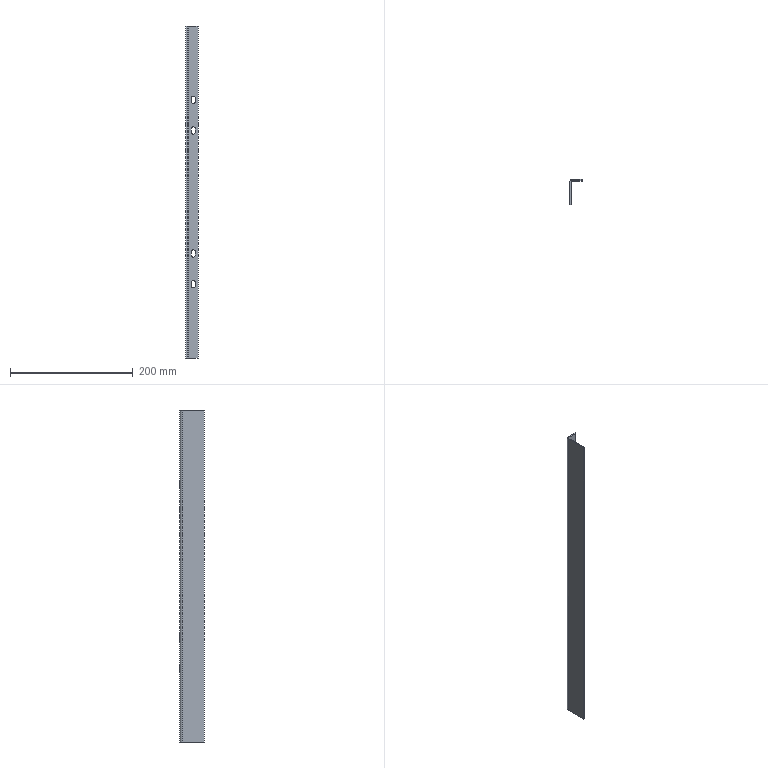Part | SolidWorks | features FlatPattern 1, ICE 1, SMBaseFlange 1, SheetMetal 1 | 1 solid | 34 faces | box 20 x 40 x 540 mm | volume 60662 mm3 | plane 20 | cylinder 14 | commonest cylinder face diameters 7 x12 4 x1 8 x1
STEP:
#1=CARTESIAN_POINT('',(12.,40.,114.));
#2=VERTEX_POINT('',#1);
#3=CARTESIAN_POINT('',(15.5,40.,117.5));
#4=VERTEX_POINT('',#3);
#5=CARTESIAN_POINT('',(12.,40.,117.5));
#6=DIRECTION('',(0.,-1.,0.));
#7=DIRECTION('',(0.,0.,-1.));
#8=AXIS2_PLACEMENT_3D('',#5,#6,#7);
#9=CIRCLE('',#8,3.5);
#10=EDGE_CURVE('',#2,#4,#9,.T.);
#11=ORIENTED_EDGE('',*,*,#10,.F.);
#12=CARTESIAN_POINT('',(12.,38.,114.));
#13=VERTEX_POINT('',#12);
#14=CARTESIAN_POINT('',(12.,40.,114.));
#15=DIRECTION('',(0.,-1.,0.));
#16=VECTOR('',#15,1000.);
#17=LINE('',#14,#16);
#18=EDGE_CURVE('',#2,#13,#17,.T.);
#19=ORIENTED_EDGE('',*,*,#18,.T.);
#20=CARTESIAN_POINT('',(15.5,38.,117.5));
#21=VERTEX_POINT('',#20);
#22=CARTESIAN_POINT('',(12.,38.,117.5));
#23=DIRECTION('',(0.,-1.,0.));
#24=DIRECTION('',(0.,0.,-1.));
#25=AXIS2_PLACEMENT_3D('',#22,#23,#24);
#26=CIRCLE('',#25,3.5);
#27=EDGE_CURVE('',#13,#21,#26,.T.);
#28=ORIENTED_EDGE('',*,*,#27,.T.);
#29=CARTESIAN_POINT('',(15.5,40.,117.5));
#30=DIRECTION('',(0.,-1.,0.));
#31=VECTOR('',#30,1000.);
#32=LINE('',#29,#31);
#33=EDGE_CURVE('',#4,#21,#32,.T.);
#34=ORIENTED_EDGE('',*,*,#33,.F.);
#35=EDGE_LOOP('',(#11,#19,#28,#34));
#36=FACE_OUTER_BOUND('',#35,.T.);
#37=CARTESIAN_POINT('',(12.,40.,117.5));
#38=DIRECTION('',(0.,-1.,0.));
#39=DIRECTION('',(0.,0.,-1.));
#40=AXIS2_PLACEMENT_3D('',#37,#38,#39);
#41=CYLINDRICAL_SURFACE('',#40,3.5);
#42=ADVANCED_FACE('',(#36),#41,.F.);
#43=CARTESIAN_POINT('',(12.,40.,164.));
#44=VERTEX_POINT('',#43);
#45=CARTESIAN_POINT('',(15.5,40.,167.5));
#46=VERTEX_POINT('',#45);
#47=CARTESIAN_POINT('',(12.,40.,167.5));
#48=DIRECTION('',(0.,-1.,0.));
#49=DIRECTION('',(0.,0.,-1.));
#50=AXIS2_PLACEMENT_3D('',#47,#48,#49);
#51=CIRCLE('',#50,3.5);
#52=EDGE_CURVE('',#44,#46,#51,.T.);
#53=ORIENTED_EDGE('',*,*,#52,.F.);
#54=CARTESIAN_POINT('',(12.,38.,164.));
#55=VERTEX_POINT('',#54);
#56=CARTESIAN_POINT('',(12.,40.,164.));
#57=DIRECTION('',(0.,-1.,0.));
#58=VECTOR('',#57,1000.);
#59=LINE('',#56,#58);
#60=EDGE_CURVE('',#44,#55,#59,.T.);
#61=ORIENTED_EDGE('',*,*,#60,.T.);
#62=CARTESIAN_POINT('',(15.5,38.,167.5));
#63=VERTEX_POINT('',#62);
#64=CARTESIAN_POINT('',(12.,38.,167.5));
#65=DIRECTION('',(0.,-1.,0.));
#66=DIRECTION('',(0.,0.,-1.));
#67=AXIS2_PLACEMENT_3D('',#64,#65,#66);
#68=CIRCLE('',#67,3.5);
#69=EDGE_CURVE('',#55,#63,#68,.T.);
#70=ORIENTED_EDGE('',*,*,#69,.T.);
#71=CARTESIAN_POINT('',(15.5,40.,167.5));
#72=DIRECTION('',(0.,-1.,0.));
#73=VECTOR('',#72,1000.);
#74=LINE('',#71,#73);
#75=EDGE_CURVE('',#46,#63,#74,.T.);
#76=ORIENTED_EDGE('',*,*,#75,.F.);
#77=EDGE_LOOP('',(#53,#61,#70,#76));
#78=FACE_OUTER_BOUND('',#77,.T.);
#79=CARTESIAN_POINT('',(12.,40.,167.5));
#80=DIRECTION('',(0.,-1.,0.));
#81=DIRECTION('',(0.,0.,-1.));
#82=AXIS2_PLACEMENT_3D('',#79,#80,#81);
#83=CYLINDRICAL_SURFACE('',#82,3.5);
#84=ADVANCED_FACE('',(#78),#83,.F.);
#85=CARTESIAN_POINT('',(12.,40.,364.));
#86=VERTEX_POINT('',#85);
#87=CARTESIAN_POINT('',(15.5,40.,367.5));
#88=VERTEX_POINT('',#87);
#89=CARTESIAN_POINT('',(12.,40.,367.5));
#90=DIRECTION('',(0.,-1.,0.));
#91=DIRECTION('',(0.,0.,1.));
#92=AXIS2_PLACEMENT_3D('',#89,#90,#91);
#93=CIRCLE('',#92,3.5);
#94=EDGE_CURVE('',#86,#88,#93,.T.);
#95=ORIENTED_EDGE('',*,*,#94,.F.);
#96=CARTESIAN_POINT('',(12.,38.,364.));
#97=VERTEX_POINT('',#96);
#98=CARTESIAN_POINT('',(12.,40.,364.));
#99=DIRECTION('',(0.,-1.,0.));
#100=VECTOR('',#99,1000.);
#101=LINE('',#98,#100);
#102=EDGE_CURVE('',#86,#97,#101,.T.);
#103=ORIENTED_EDGE('',*,*,#102,.T.);
#104=CARTESIAN_POINT('',(15.5,38.,367.5));
#105=VERTEX_POINT('',#104);
#106=CARTESIAN_POINT('',(12.,38.,367.5));
#107=DIRECTION('',(0.,-1.,0.));
#108=DIRECTION('',(0.,0.,1.));
#109=AXIS2_PLACEMENT_3D('',#106,#107,#108);
#110=CIRCLE('',#109,3.5);
#111=EDGE_CURVE('',#97,#105,#110,.T.);
#112=ORIENTED_EDGE('',*,*,#111,.T.);
#113=CARTESIAN_POINT('',(15.5,40.,367.5));
#114=DIRECTION('',(0.,-1.,0.));
#115=VECTOR('',#114,1000.);
#116=LINE('',#113,#115);
#117=EDGE_CURVE('',#88,#105,#116,.T.);
#118=ORIENTED_EDGE('',*,*,#117,.F.);
#119=EDGE_LOOP('',(#95,#103,#112,#118));
#120=FACE_OUTER_BOUND('',#119,.T.);
#121=CARTESIAN_POINT('',(12.,40.,367.5));
#122=DIRECTION('',(0.,-1.,0.));
#123=DIRECTION('',(0.,0.,-1.));
#124=AXIS2_PLACEMENT_3D('',#121,#122,#123);
#125=CYLINDRICAL_SURFACE('',#124,3.5);
#126=ADVANCED_FACE('',(#120),#125,.F.);
#127=CARTESIAN_POINT('',(12.,40.,414.));
#128=VERTEX_POINT('',#127);
#129=CARTESIAN_POINT('',(15.5,40.,417.5));
#130=VERTEX_POINT('',#129);
#131=CARTESIAN_POINT('',(12.,40.,417.5));
#132=DIRECTION('',(0.,-1.,0.));
#133=DIRECTION('',(0.,0.,1.));
#134=AXIS2_PLACEMENT_3D('',#131,#132,#133);
#135=CIRCLE('',#134,3.5);
#136=EDGE_CURVE('',#128,#130,#135,.T.);
#137=ORIENTED_EDGE('',*,*,#136,.F.);
#138=CARTESIAN_POINT('',(12.,38.,414.));
#139=VERTEX_POINT('',#138);
#140=CARTESIAN_POINT('',(12.,40.,414.));
#141=DIRECTION('',(0.,-1.,0.));
#142=VECTOR('',#141,1000.);
#143=LINE('',#140,#142);
#144=EDGE_CURVE('',#128,#139,#143,.T.);
#145=ORIENTED_EDGE('',*,*,#144,.T.);
#146=CARTESIAN_POINT('',(15.5,38.,417.5));
#147=VERTEX_POINT('',#146);
#148=CARTESIAN_POINT('',(12.,38.,417.5));
#149=DIRECTION('',(0.,-1.,0.));
#150=DIRECTION('',(0.,0.,1.));
#151=AXIS2_PLACEMENT_3D('',#148,#149,#150);
#152=CIRCLE('',#151,3.5);
#153=EDGE_CURVE('',#139,#147,#152,.T.);
#154=ORIENTED_EDGE('',*,*,#153,.T.);
#155=CARTESIAN_POINT('',(15.5,40.,417.5));
#156=DIRECTION('',(0.,-1.,0.));
#157=VECTOR('',#156,1000.);
#158=LINE('',#155,#157);
#159=EDGE_CURVE('',#130,#147,#158,.T.);
#160=ORIENTED_EDGE('',*,*,#159,.F.);
#161=EDGE_LOOP('',(#137,#145,#154,#160));
#162=FACE_OUTER_BOUND('',#161,.T.);
#163=CARTESIAN_POINT('',(12.,40.,417.5));
#164=DIRECTION('',(0.,-1.,0.));
#165=DIRECTION('',(0.,0.,-1.));
#166=AXIS2_PLACEMENT_3D('',#163,#164,#165);
#167=CYLINDRICAL_SURFACE('',#166,3.5);
#168=ADVANCED_FACE('',(#162),#167,.F.);
#169=CARTESIAN_POINT('',(4.,40.,540.));
#170=VERTEX_POINT('',#169);
#171=CARTESIAN_POINT('',(4.,38.,540.));
#172=VERTEX_POINT('',#171);
#173=CARTESIAN_POINT('',(4.,40.,540.));
#174=DIRECTION('',(0.,-1.,0.));
#175=VECTOR('',#174,1000.);
#176=LINE('',#173,#175);
#177=EDGE_CURVE('',#170,#172,#176,.T.);
#178=ORIENTED_EDGE('',*,*,#177,.F.);
#179=CARTESIAN_POINT('',(0.,36.,540.));
#180=VERTEX_POINT('',#179);
#181=CARTESIAN_POINT('',(4.,36.,540.));
#182=DIRECTION('',(0.,0.,-1.));
#183=DIRECTION('',(1.,0.,0.));
#184=AXIS2_PLACEMENT_3D('',#181,#182,#183);
#185=CIRCLE('',#184,4.);
#186=EDGE_CURVE('',#180,#170,#185,.T.);
#187=ORIENTED_EDGE('',*,*,#186,.F.);
#188=CARTESIAN_POINT('',(2.,36.,540.));
#189=VERTEX_POINT('',#188);
#190=CARTESIAN_POINT('',(2.,36.,540.));
#191=DIRECTION('',(-1.,0.,0.));
#192=VECTOR('',#191,1000.);
#193=LINE('',#190,#192);
#194=EDGE_CURVE('',#189,#180,#193,.T.);
#195=ORIENTED_EDGE('',*,*,#194,.F.);
#196=CARTESIAN_POINT('',(4.,36.,540.));
#197=DIRECTION('',(0.,0.,-1.));
#198=DIRECTION('',(1.,0.,0.));
#199=AXIS2_PLACEMENT_3D('',#196,#197,#198);
#200=CIRCLE('',#199,2.);
#201=EDGE_CURVE('',#189,#172,#200,.T.);
#202=ORIENTED_EDGE('',*,*,#201,.T.);
#203=EDGE_LOOP('',(#178,#187,#195,#202));
#204=FACE_OUTER_BOUND('',#203,.T.);
#205=CARTESIAN_POINT('',(4.,40.,540.));
#206=DIRECTION('',(0.,0.,1.));
#207=DIRECTION('',(1.,0.,0.));
#208=AXIS2_PLACEMENT_3D('',#205,#206,#207);
#209=PLANE('',#208);
#210=ADVANCED_FACE('',(#204),#209,.T.);
#211=CARTESIAN_POINT('',(20.,40.,540.));
#212=VERTEX_POINT('',#211);
#213=CARTESIAN_POINT('',(0.,40.,540.));
#214=DIRECTION('',(1.,0.,0.));
#215=VECTOR('',#214,1000.);
#216=LINE('',#213,#215);
#217=EDGE_CURVE('',#170,#212,#216,.T.);
#218=ORIENTED_EDGE('',*,*,#217,.F.);
#219=ORIENTED_EDGE('',*,*,#177,.T.);
#220=CARTESIAN_POINT('',(20.,38.,540.));
#221=VERTEX_POINT('',#220);
#222=CARTESIAN_POINT('',(0.,38.,540.));
#223=DIRECTION('',(1.,0.,0.));
#224=VECTOR('',#223,1000.);
#225=LINE('',#222,#224);
#226=EDGE_CURVE('',#172,#221,#225,.T.);
#227=ORIENTED_EDGE('',*,*,#226,.T.);
#228=CARTESIAN_POINT('',(20.,40.,540.));
#229=DIRECTION('',(0.,-1.,0.));
#230=VECTOR('',#229,1000.);
#231=LINE('',#228,#230);
#232=EDGE_CURVE('',#212,#221,#231,.T.);
#233=ORIENTED_EDGE('',*,*,#232,.F.);
#234=EDGE_LOOP('',(#218,#219,#227,#233));
#235=FACE_OUTER_BOUND('',#234,.T.);
#236=CARTESIAN_POINT('',(2.,36.,540.));
#237=DIRECTION('',(0.,0.,1.));
#238=DIRECTION('',(1.,0.,0.));
#239=AXIS2_PLACEMENT_3D('',#236,#237,#238);
#240=PLANE('',#239);
#241=ADVANCED_FACE('',(#235),#240,.T.);
#242=CARTESIAN_POINT('',(0.,36.,0.));
#243=VERTEX_POINT('',#242);
#244=CARTESIAN_POINT('',(2.,36.,0.));
#245=VERTEX_POINT('',#244);
#246=CARTESIAN_POINT('',(0.,36.,0.));
#247=DIRECTION('',(1.,0.,0.));
#248=VECTOR('',#247,1000.);
#249=LINE('',#246,#248);
#250=EDGE_CURVE('',#243,#245,#249,.T.);
#251=ORIENTED_EDGE('',*,*,#250,.F.);
#252=CARTESIAN_POINT('',(4.,40.,0.));
#253=VERTEX_POINT('',#252);
#254=CARTESIAN_POINT('',(4.,36.,0.));
#255=DIRECTION('',(0.,0.,-1.));
#256=DIRECTION('',(1.,0.,0.));
#257=AXIS2_PLACEMENT_3D('',#254,#255,#256);
#258=CIRCLE('',#257,4.);
#259=EDGE_CURVE('',#243,#253,#258,.T.);
#260=ORIENTED_EDGE('',*,*,#259,.T.);
#261=CARTESIAN_POINT('',(4.,38.,0.));
#262=VERTEX_POINT('',#261);
#263=CARTESIAN_POINT('',(4.,38.,0.));
#264=DIRECTION('',(0.,1.,0.));
#265=VECTOR('',#264,1000.);
#266=LINE('',#263,#265);
#267=EDGE_CURVE('',#262,#253,#266,.T.);
#268=ORIENTED_EDGE('',*,*,#267,.F.);
#269=CARTESIAN_POINT('',(4.,36.,0.));
#270=DIRECTION('',(0.,0.,-1.));
#271=DIRECTION('',(1.,0.,0.));
#272=AXIS2_PLACEMENT_3D('',#269,#270,#271);
#273=CIRCLE('',#272,2.);
#274=EDGE_CURVE('',#245,#262,#273,.T.);
#275=ORIENTED_EDGE('',*,*,#274,.F.);
#276=EDGE_LOOP('',(#251,#260,#268,#275));
#277=FACE_OUTER_BOUND('',#276,.T.);
#278=CARTESIAN_POINT('',(0.,36.,0.));
#279=DIRECTION('',(0.,0.,-1.));
#280=DIRECTION('',(-1.,0.,0.));
#281=AXIS2_PLACEMENT_3D('',#278,#279,#280);
#282=PLANE('',#281);
#283=ADVANCED_FACE('',(#277),#282,.T.);
#284=CARTESIAN_POINT('',(0.,0.,0.));
#285=VERTEX_POINT('',#284);
#286=CARTESIAN_POINT('',(0.,0.,0.));
#287=DIRECTION('',(0.,1.,0.));
#288=VECTOR('',#287,1000.);
#289=LINE('',#286,#288);
#290=EDGE_CURVE('',#285,#243,#289,.T.);
#291=ORIENTED_EDGE('',*,*,#290,.T.);
#292=ORIENTED_EDGE('',*,*,#250,.T.);
#293=CARTESIAN_POINT('',(2.,0.,0.));
#294=VERTEX_POINT('',#293);
#295=CARTESIAN_POINT('',(2.,0.,0.));
#296=DIRECTION('',(0.,1.,0.));
#297=VECTOR('',#296,1000.);
#298=LINE('',#295,#297);
#299=EDGE_CURVE('',#294,#245,#298,.T.);
#300=ORIENTED_EDGE('',*,*,#299,.F.);
#301=CARTESIAN_POINT('',(2.,0.,0.));
#302=DIRECTION('',(-1.,0.,0.));
#303=VECTOR('',#302,1000.);
#304=LINE('',#301,#303);
#305=EDGE_CURVE('',#294,#285,#304,.T.);
#306=ORIENTED_EDGE('',*,*,#305,.T.);
#307=EDGE_LOOP('',(#291,#292,#300,#306));
#308=FACE_OUTER_BOUND('',#307,.T.);
#309=CARTESIAN_POINT('',(4.,38.,0.));
#310=DIRECTION('',(0.,0.,-1.));
#311=DIRECTION('',(-1.,0.,0.));
#312=AXIS2_PLACEMENT_3D('',#309,#310,#311);
#313=PLANE('',#312);
#314=ADVANCED_FACE('',(#308),#313,.T.);
#315=CARTESIAN_POINT('',(15.5,38.,122.5));
#316=VERTEX_POINT('',#315);
#317=CARTESIAN_POINT('',(15.5,38.,117.5));
#318=DIRECTION('',(0.,0.,1.));
#319=VECTOR('',#318,1000.);
#320=LINE('',#317,#319);
#321=EDGE_CURVE('',#21,#316,#320,.T.);
#322=ORIENTED_EDGE('',*,*,#321,.F.);
#323=ORIENTED_EDGE('',*,*,#27,.F.);
#324=CARTESIAN_POINT('',(8.5,38.,117.5));
#325=VERTEX_POINT('',#324);
#326=CARTESIAN_POINT('',(12.,38.,117.5));
#327=DIRECTION('',(0.,-1.,0.));
#328=DIRECTION('',(0.,0.,-1.));
#329=AXIS2_PLACEMENT_3D('',#326,#327,#328);
#330=CIRCLE('',#329,3.5);
#331=EDGE_CURVE('',#325,#13,#330,.T.);
#332=ORIENTED_EDGE('',*,*,#331,.F.);
#333=CARTESIAN_POINT('',(8.5,38.,122.5));
#334=VERTEX_POINT('',#333);
#335=CARTESIAN_POINT('',(8.5,38.,117.5));
#336=DIRECTION('',(0.,0.,-1.));
#337=VECTOR('',#336,1000.);
#338=LINE('',#335,#337);
#339=EDGE_CURVE('',#334,#325,#338,.T.);
#340=ORIENTED_EDGE('',*,*,#339,.F.);
#341=CARTESIAN_POINT('',(12.,38.,122.5));
#342=DIRECTION('',(0.,-1.,0.));
#343=DIRECTION('',(0.,0.,-1.));
#344=AXIS2_PLACEMENT_3D('',#341,#342,#343);
#345=CIRCLE('',#344,3.5);
#346=EDGE_CURVE('',#316,#334,#345,.T.);
#347=ORIENTED_EDGE('',*,*,#346,.F.);
#348=EDGE_LOOP('',(#322,#323,#332,#340,#347));
#349=FACE_BOUND('',#348,.T.);
#350=CARTESIAN_POINT('',(15.5,38.,172.5));
#351=VERTEX_POINT('',#350);
#352=CARTESIAN_POINT('',(15.5,38.,167.5));
#353=DIRECTION('',(0.,0.,1.));
#354=VECTOR('',#353,1000.);
#355=LINE('',#352,#354);
#356=EDGE_CURVE('',#63,#351,#355,.T.);
#357=ORIENTED_EDGE('',*,*,#356,.F.);
#358=ORIENTED_EDGE('',*,*,#69,.F.);
#359=CARTESIAN_POINT('',(8.5,38.,167.5));
#360=VERTEX_POINT('',#359);
#361=CARTESIAN_POINT('',(12.,38.,167.5));
#362=DIRECTION('',(0.,-1.,0.));
#363=DIRECTION('',(0.,0.,-1.));
#364=AXIS2_PLACEMENT_3D('',#361,#362,#363);
#365=CIRCLE('',#364,3.5);
#366=EDGE_CURVE('',#360,#55,#365,.T.);
#367=ORIENTED_EDGE('',*,*,#366,.F.);
#368=CARTESIAN_POINT('',(8.5,38.,172.5));
#369=VERTEX_POINT('',#368);
#370=CARTESIAN_POINT('',(8.5,38.,167.5));
#371=DIRECTION('',(0.,0.,-1.));
#372=VECTOR('',#371,1000.);
#373=LINE('',#370,#372);
#374=EDGE_CURVE('',#369,#360,#373,.T.);
#375=ORIENTED_EDGE('',*,*,#374,.F.);
#376=CARTESIAN_POINT('',(12.,38.,172.5));
#377=DIRECTION('',(0.,-1.,0.));
#378=DIRECTION('',(0.,0.,-1.));
#379=AXIS2_PLACEMENT_3D('',#376,#377,#378);
#380=CIRCLE('',#379,3.5);
#381=EDGE_CURVE('',#351,#369,#380,.T.);
#382=ORIENTED_EDGE('',*,*,#381,.F.);
#383=EDGE_LOOP('',(#357,#358,#367,#375,#382));
#384=FACE_BOUND('',#383,.T.);
#385=CARTESIAN_POINT('',(8.5,38.,372.5));
#386=VERTEX_POINT('',#385);
#387=CARTESIAN_POINT('',(8.5,38.,367.5));
#388=VERTEX_POINT('',#387);
#389=CARTESIAN_POINT('',(8.5,38.,372.5));
#390=DIRECTION('',(0.,0.,-1.));
#391=VECTOR('',#390,1000.);
#392=LINE('',#389,#391);
#393=EDGE_CURVE('',#386,#388,#392,.T.);
#394=ORIENTED_EDGE('',*,*,#393,.F.);
#395=CARTESIAN_POINT('',(15.5,38.,372.5));
#396=VERTEX_POINT('',#395);
#397=CARTESIAN_POINT('',(12.,38.,372.5));
#398=DIRECTION('',(0.,-1.,0.));
#399=DIRECTION('',(0.,0.,1.));
#400=AXIS2_PLACEMENT_3D('',#397,#398,#399);
#401=CIRCLE('',#400,3.5);
#402=EDGE_CURVE('',#396,#386,#401,.T.);
#403=ORIENTED_EDGE('',*,*,#402,.F.);
#404=CARTESIAN_POINT('',(15.5,38.,372.5));
#405=DIRECTION('',(0.,0.,1.));
#406=VECTOR('',#405,1000.);
#407=LINE('',#404,#406);
#408=EDGE_CURVE('',#105,#396,#407,.T.);
#409=ORIENTED_EDGE('',*,*,#408,.F.);
#410=ORIENTED_EDGE('',*,*,#111,.F.);
#411=CARTESIAN_POINT('',(12.,38.,367.5));
#412=DIRECTION('',(0.,-1.,0.));
#413=DIRECTION('',(0.,0.,1.));
#414=AXIS2_PLACEMENT_3D('',#411,#412,#413);
#415=CIRCLE('',#414,3.5);
#416=EDGE_CURVE('',#388,#97,#415,.T.);
#417=ORIENTED_EDGE('',*,*,#416,.F.);
#418=EDGE_LOOP('',(#394,#403,#409,#410,#417));
#419=FACE_BOUND('',#418,.T.);
#420=CARTESIAN_POINT('',(8.5,38.,422.5));
#421=VERTEX_POINT('',#420);
#422=CARTESIAN_POINT('',(8.5,38.,417.5));
#423=VERTEX_POINT('',#422);
#424=CARTESIAN_POINT('',(8.5,38.,422.5));
#425=DIRECTION('',(0.,0.,-1.));
#426=VECTOR('',#425,1000.);
#427=LINE('',#424,#426);
#428=EDGE_CURVE('',#421,#423,#427,.T.);
#429=ORIENTED_EDGE('',*,*,#428,.F.);
#430=CARTESIAN_POINT('',(15.5,38.,422.5));
#431=VERTEX_POINT('',#430);
#432=CARTESIAN_POINT('',(12.,38.,422.5));
#433=DIRECTION('',(0.,-1.,0.));
#434=DIRECTION('',(0.,0.,1.));
#435=AXIS2_PLACEMENT_3D('',#432,#433,#434);
#436=CIRCLE('',#435,3.5);
#437=EDGE_CURVE('',#431,#421,#436,.T.);
#438=ORIENTED_EDGE('',*,*,#437,.F.);
#439=CARTESIAN_POINT('',(15.5,38.,422.5));
#440=DIRECTION('',(0.,0.,1.));
#441=VECTOR('',#440,1000.);
#442=LINE('',#439,#441);
#443=EDGE_CURVE('',#147,#431,#442,.T.);
#444=ORIENTED_EDGE('',*,*,#443,.F.);
#445=ORIENTED_EDGE('',*,*,#153,.F.);
#446=CARTESIAN_POINT('',(12.,38.,417.5));
#447=DIRECTION('',(0.,-1.,0.));
#448=DIRECTION('',(0.,0.,1.));
#449=AXIS2_PLACEMENT_3D('',#446,#447,#448);
#450=CIRCLE('',#449,3.5);
#451=EDGE_CURVE('',#423,#139,#450,.T.);
#452=ORIENTED_EDGE('',*,*,#451,.F.);
#453=EDGE_LOOP('',(#429,#438,#444,#445,#452));
#454=FACE_BOUND('',#453,.T.);
#455=CARTESIAN_POINT('',(20.,38.,0.));
#456=VERTEX_POINT('',#455);
#457=CARTESIAN_POINT('',(0.,38.,0.));
#458=DIRECTION('',(1.,0.,0.));
#459=VECTOR('',#458,1000.);
#460=LINE('',#457,#459);
#461=EDGE_CURVE('',#262,#456,#460,.T.);
#462=ORIENTED_EDGE('',*,*,#461,.T.);
#463=CARTESIAN_POINT('',(20.,38.,540.));
#464=DIRECTION('',(0.,0.,-1.));
#465=VECTOR('',#464,1000.);
#466=LINE('',#463,#465);
#467=EDGE_CURVE('',#221,#456,#466,.T.);
#468=ORIENTED_EDGE('',*,*,#467,.F.);
#469=ORIENTED_EDGE('',*,*,#226,.F.);
#470=CARTESIAN_POINT('',(4.,38.,540.));
#471=DIRECTION('',(0.,0.,-1.));
#472=VECTOR('',#471,1000.);
#473=LINE('',#470,#472);
#474=EDGE_CURVE('',#172,#262,#473,.T.);
#475=ORIENTED_EDGE('',*,*,#474,.T.);
#476=EDGE_LOOP('',(#462,#468,#469,#475));
#477=FACE_OUTER_BOUND('',#476,.T.);
#478=CARTESIAN_POINT('',(0.,38.,540.));
#479=DIRECTION('',(0.,1.,0.));
#480=DIRECTION('',(0.,0.,1.));
#481=AXIS2_PLACEMENT_3D('',#478,#479,#480);
#482=PLANE('',#481);
#483=ADVANCED_FACE('',(#349,#384,#419,#454,#477),#482,.F.);
#484=CARTESIAN_POINT('',(20.,40.,0.));
#485=VERTEX_POINT('',#484);
#486=CARTESIAN_POINT('',(20.,40.,0.));
#487=DIRECTION('',(0.,-1.,0.));
#488=VECTOR('',#487,1000.);
#489=LINE('',#486,#488);
#490=EDGE_CURVE('',#485,#456,#489,.T.);
#491=ORIENTED_EDGE('',*,*,#490,.F.);
#492=CARTESIAN_POINT('',(20.,40.,540.));
#493=DIRECTION('',(0.,0.,-1.));
#494=VECTOR('',#493,1000.);
#495=LINE('',#492,#494);
#496=EDGE_CURVE('',#212,#485,#495,.T.);
#497=ORIENTED_EDGE('',*,*,#496,.F.);
#498=ORIENTED_EDGE('',*,*,#232,.T.);
#499=ORIENTED_EDGE('',*,*,#467,.T.);
#500=EDGE_LOOP('',(#491,#497,#498,#499));
#501=FACE_OUTER_BOUND('',#500,.T.);
#502=CARTESIAN_POINT('',(20.,40.,540.));
#503=DIRECTION('',(1.,0.,0.));
#504=DIRECTION('',(0.,0.,-1.));
#505=AXIS2_PLACEMENT_3D('',#502,#503,#504);
#506=PLANE('',#505);
#507=ADVANCED_FACE('',(#501),#506,.T.);
#508=CARTESIAN_POINT('',(8.5,40.,117.5));
#509=VERTEX_POINT('',#508);
#510=CARTESIAN_POINT('',(12.,40.,117.5));
#511=DIRECTION('',(0.,-1.,0.));
#512=DIRECTION('',(0.,0.,-1.));
#513=AXIS2_PLACEMENT_3D('',#510,#511,#512);
#514=CIRCLE('',#513,3.5);
#515=EDGE_CURVE('',#509,#2,#514,.T.);
#516=ORIENTED_EDGE('',*,*,#515,.T.);
#517=ORIENTED_EDGE('',*,*,#10,.T.);
#518=CARTESIAN_POINT('',(15.5,40.,122.5));
#519=VERTEX_POINT('',#518);
#520=CARTESIAN_POINT('',(15.5,40.,117.5));
#521=DIRECTION('',(0.,0.,1.));
#522=VECTOR('',#521,1000.);
#523=LINE('',#520,#522);
#524=EDGE_CURVE('',#4,#519,#523,.T.);
#525=ORIENTED_EDGE('',*,*,#524,.T.);
#526=CARTESIAN_POINT('',(8.5,40.,122.5));
#527=VERTEX_POINT('',#526);
#528=CARTESIAN_POINT('',(12.,40.,122.5));
#529=DIRECTION('',(0.,-1.,0.));
#530=DIRECTION('',(0.,0.,-1.));
#531=AXIS2_PLACEMENT_3D('',#528,#529,#530);
#532=CIRCLE('',#531,3.5);
#533=EDGE_CURVE('',#519,#527,#532,.T.);
#534=ORIENTED_EDGE('',*,*,#533,.T.);
#535=CARTESIAN_POINT('',(8.5,40.,117.5));
#536=DIRECTION('',(0.,0.,-1.));
#537=VECTOR('',#536,1000.);
#538=LINE('',#535,#537);
#539=EDGE_CURVE('',#527,#509,#538,.T.);
#540=ORIENTED_EDGE('',*,*,#539,.T.);
#541=EDGE_LOOP('',(#516,#517,#525,#534,#540));
#542=FACE_BOUND('',#541,.T.);
#543=CARTESIAN_POINT('',(8.5,40.,167.5));
#544=VERTEX_POINT('',#543);
#545=CARTESIAN_POINT('',(12.,40.,167.5));
#546=DIRECTION('',(0.,-1.,0.));
#547=DIRECTION('',(0.,0.,-1.));
#548=AXIS2_PLACEMENT_3D('',#545,#546,#547);
#549=CIRCLE('',#548,3.5);
#550=EDGE_CURVE('',#544,#44,#549,.T.);
#551=ORIENTED_EDGE('',*,*,#550,.T.);
#552=ORIENTED_EDGE('',*,*,#52,.T.);
#553=CARTESIAN_POINT('',(15.5,40.,172.5));
#554=VERTEX_POINT('',#553);
#555=CARTESIAN_POINT('',(15.5,40.,167.5));
#556=DIRECTION('',(0.,0.,1.));
#557=VECTOR('',#556,1000.);
#558=LINE('',#555,#557);
#559=EDGE_CURVE('',#46,#554,#558,.T.);
#560=ORIENTED_EDGE('',*,*,#559,.T.);
#561=CARTESIAN_POINT('',(8.5,40.,172.5));
#562=VERTEX_POINT('',#561);
#563=CARTESIAN_POINT('',(12.,40.,172.5));
#564=DIRECTION('',(0.,-1.,0.));
#565=DIRECTION('',(0.,0.,-1.));
#566=AXIS2_PLACEMENT_3D('',#563,#564,#565);
#567=CIRCLE('',#566,3.5);
#568=EDGE_CURVE('',#554,#562,#567,.T.);
#569=ORIENTED_EDGE('',*,*,#568,.T.);
#570=CARTESIAN_POINT('',(8.5,40.,167.5));
#571=DIRECTION('',(0.,0.,-1.));
#572=VECTOR('',#571,1000.);
#573=LINE('',#570,#572);
#574=EDGE_CURVE('',#562,#544,#573,.T.);
#575=ORIENTED_EDGE('',*,*,#574,.T.);
#576=EDGE_LOOP('',(#551,#552,#560,#569,#575));
#577=FACE_BOUND('',#576,.T.);
#578=CARTESIAN_POINT('',(15.5,40.,372.5));
#579=VERTEX_POINT('',#578);
#580=CARTESIAN_POINT('',(8.5,40.,372.5));
#581=VERTEX_POINT('',#580);
#582=CARTESIAN_POINT('',(12.,40.,372.5));
#583=DIRECTION('',(0.,-1.,0.));
#584=DIRECTION('',(0.,0.,1.));
#585=AXIS2_PLACEMENT_3D('',#582,#583,#584);
#586=CIRCLE('',#585,3.5);
#587=EDGE_CURVE('',#579,#581,#586,.T.);
#588=ORIENTED_EDGE('',*,*,#587,.T.);
#589=CARTESIAN_POINT('',(8.5,40.,367.5));
#590=VERTEX_POINT('',#589);
#591=CARTESIAN_POINT('',(8.5,40.,372.5));
#592=DIRECTION('',(0.,0.,-1.));
#593=VECTOR('',#592,1000.);
#594=LINE('',#591,#593);
#595=EDGE_CURVE('',#581,#590,#594,.T.);
#596=ORIENTED_EDGE('',*,*,#595,.T.);
#597=CARTESIAN_POINT('',(12.,40.,367.5));
#598=DIRECTION('',(0.,-1.,0.));
#599=DIRECTION('',(0.,0.,1.));
#600=AXIS2_PLACEMENT_3D('',#597,#598,#599);
#601=CIRCLE('',#600,3.5);
#602=EDGE_CURVE('',#590,#86,#601,.T.);
#603=ORIENTED_EDGE('',*,*,#602,.T.);
#604=ORIENTED_EDGE('',*,*,#94,.T.);
#605=CARTESIAN_POINT('',(15.5,40.,372.5));
#606=DIRECTION('',(0.,0.,1.));
#607=VECTOR('',#606,1000.);
#608=LINE('',#605,#607);
#609=EDGE_CURVE('',#88,#579,#608,.T.);
#610=ORIENTED_EDGE('',*,*,#609,.T.);
#611=EDGE_LOOP('',(#588,#596,#603,#604,#610));
#612=FACE_BOUND('',#611,.T.);
#613=CARTESIAN_POINT('',(15.5,40.,422.5));
#614=VERTEX_POINT('',#613);
#615=CARTESIAN_POINT('',(8.5,40.,422.5));
#616=VERTEX_POINT('',#615);
#617=CARTESIAN_POINT('',(12.,40.,422.5));
#618=DIRECTION('',(0.,-1.,0.));
#619=DIRECTION('',(0.,0.,1.));
#620=AXIS2_PLACEMENT_3D('',#617,#618,#619);
#621=CIRCLE('',#620,3.5);
#622=EDGE_CURVE('',#614,#616,#621,.T.);
#623=ORIENTED_EDGE('',*,*,#622,.T.);
#624=CARTESIAN_POINT('',(8.5,40.,417.5));
#625=VERTEX_POINT('',#624);
#626=CARTESIAN_POINT('',(8.5,40.,422.5));
#627=DIRECTION('',(0.,0.,-1.));
#628=VECTOR('',#627,1000.);
#629=LINE('',#626,#628);
#630=EDGE_CURVE('',#616,#625,#629,.T.);
#631=ORIENTED_EDGE('',*,*,#630,.T.);
#632=CARTESIAN_POINT('',(12.,40.,417.5));
#633=DIRECTION('',(0.,-1.,0.));
#634=DIRECTION('',(0.,0.,1.));
#635=AXIS2_PLACEMENT_3D('',#632,#633,#634);
#636=CIRCLE('',#635,3.5);
#637=EDGE_CURVE('',#625,#128,#636,.T.);
#638=ORIENTED_EDGE('',*,*,#637,.T.);
#639=ORIENTED_EDGE('',*,*,#136,.T.);
#640=CARTESIAN_POINT('',(15.5,40.,422.5));
#641=DIRECTION('',(0.,0.,1.));
#642=VECTOR('',#641,1000.);
#643=LINE('',#640,#642);
#644=EDGE_CURVE('',#130,#614,#643,.T.);
#645=ORIENTED_EDGE('',*,*,#644,.T.);
#646=EDGE_LOOP('',(#623,#631,#638,#639,#645));
#647=FACE_BOUND('',#646,.T.);
#648=CARTESIAN_POINT('',(0.,40.,0.));
#649=DIRECTION('',(1.,0.,0.));
#650=VECTOR('',#649,1000.);
#651=LINE('',#648,#650);
#652=EDGE_CURVE('',#253,#485,#651,.T.);
#653=ORIENTED_EDGE('',*,*,#652,.F.);
#654=CARTESIAN_POINT('',(4.,40.,540.));
#655=DIRECTION('',(0.,0.,-1.));
#656=VECTOR('',#655,1000.);
#657=LINE('',#654,#656);
#658=EDGE_CURVE('',#170,#253,#657,.T.);
#659=ORIENTED_EDGE('',*,*,#658,.F.);
#660=ORIENTED_EDGE('',*,*,#217,.T.);
#661=ORIENTED_EDGE('',*,*,#496,.T.);
#662=EDGE_LOOP('',(#653,#659,#660,#661));
#663=FACE_OUTER_BOUND('',#662,.T.);
#664=CARTESIAN_POINT('',(0.,40.,540.));
#665=DIRECTION('',(0.,1.,0.));
#666=DIRECTION('',(0.,0.,1.));
#667=AXIS2_PLACEMENT_3D('',#664,#665,#666);
#668=PLANE('',#667);
#669=ADVANCED_FACE('',(#542,#577,#612,#647,#663),#668,.T.);
#670=ORIENTED_EDGE('',*,*,#259,.F.);
#671=CARTESIAN_POINT('',(0.,36.,540.));
#672=DIRECTION('',(0.,0.,-1.));
#673=VECTOR('',#672,1000.);
#674=LINE('',#671,#673);
#675=EDGE_CURVE('',#180,#243,#674,.T.);
#676=ORIENTED_EDGE('',*,*,#675,.F.);
#677=ORIENTED_EDGE('',*,*,#186,.T.);
#678=ORIENTED_EDGE('',*,*,#658,.T.);
#679=EDGE_LOOP('',(#670,#676,#677,#678));
#680=FACE_OUTER_BOUND('',#679,.T.);
#681=CARTESIAN_POINT('',(4.,36.,540.));
#682=DIRECTION('',(0.,0.,-1.));
#683=DIRECTION('',(-1.,0.,0.));
#684=AXIS2_PLACEMENT_3D('',#681,#682,#683);
#685=CYLINDRICAL_SURFACE('',#684,4.);
#686=ADVANCED_FACE('',(#680),#685,.T.);
#687=ORIENTED_EDGE('',*,*,#290,.F.);
#688=CARTESIAN_POINT('',(0.,0.,540.));
#689=VERTEX_POINT('',#688);
#690=CARTESIAN_POINT('',(0.,0.,540.));
#691=DIRECTION('',(0.,0.,-1.));
#692=VECTOR('',#691,1000.);
#693=LINE('',#690,#692);
#694=EDGE_CURVE('',#689,#285,#693,.T.);
#695=ORIENTED_EDGE('',*,*,#694,.F.);
#696=CARTESIAN_POINT('',(0.,0.,540.));
#697=DIRECTION('',(0.,1.,0.));
#698=VECTOR('',#697,1000.);
#699=LINE('',#696,#698);
#700=EDGE_CURVE('',#689,#180,#699,.T.);
#701=ORIENTED_EDGE('',*,*,#700,.T.);
#702=ORIENTED_EDGE('',*,*,#675,.T.);
#703=EDGE_LOOP('',(#687,#695,#701,#702));
#704=FACE_OUTER_BOUND('',#703,.T.);
#705=CARTESIAN_POINT('',(0.,0.,540.));
#706=DIRECTION('',(-1.,0.,0.));
#707=DIRECTION('',(0.,0.,1.));
#708=AXIS2_PLACEMENT_3D('',#705,#706,#707);
#709=PLANE('',#708);
#710=ADVANCED_FACE('',(#704),#709,.T.);
#711=ORIENTED_EDGE('',*,*,#305,.F.);
#712=CARTESIAN_POINT('',(2.,0.,540.));
#713=VERTEX_POINT('',#712);
#714=CARTESIAN_POINT('',(2.,0.,540.));
#715=DIRECTION('',(0.,0.,-1.));
#716=VECTOR('',#715,1000.);
#717=LINE('',#714,#716);
#718=EDGE_CURVE('',#713,#294,#717,.T.);
#719=ORIENTED_EDGE('',*,*,#718,.F.);
#720=CARTESIAN_POINT('',(2.,0.,540.));
#721=DIRECTION('',(-1.,0.,0.));
#722=VECTOR('',#721,1000.);
#723=LINE('',#720,#722);
#724=EDGE_CURVE('',#713,#689,#723,.T.);
#725=ORIENTED_EDGE('',*,*,#724,.T.);
#726=ORIENTED_EDGE('',*,*,#694,.T.);
#727=EDGE_LOOP('',(#711,#719,#725,#726));
#728=FACE_OUTER_BOUND('',#727,.T.);
#729=CARTESIAN_POINT('',(2.,0.,540.));
#730=DIRECTION('',(0.,-1.,0.));
#731=DIRECTION('',(0.,0.,-1.));
#732=AXIS2_PLACEMENT_3D('',#729,#730,#731);
#733=PLANE('',#732);
#734=ADVANCED_FACE('',(#728),#733,.T.);
#735=ORIENTED_EDGE('',*,*,#299,.T.);
#736=CARTESIAN_POINT('',(2.,36.,540.));
#737=DIRECTION('',(0.,0.,-1.));
#738=VECTOR('',#737,1000.);
#739=LINE('',#736,#738);
#740=EDGE_CURVE('',#189,#245,#739,.T.);
#741=ORIENTED_EDGE('',*,*,#740,.F.);
#742=CARTESIAN_POINT('',(2.,0.,540.));
#743=DIRECTION('',(0.,1.,0.));
#744=VECTOR('',#743,1000.);
#745=LINE('',#742,#744);
#746=EDGE_CURVE('',#713,#189,#745,.T.);
#747=ORIENTED_EDGE('',*,*,#746,.F.);
#748=ORIENTED_EDGE('',*,*,#718,.T.);
#749=EDGE_LOOP('',(#735,#741,#747,#748));
#750=FACE_OUTER_BOUND('',#749,.T.);
#751=CARTESIAN_POINT('',(2.,0.,540.));
#752=DIRECTION('',(-1.,0.,0.));
#753=DIRECTION('',(0.,0.,1.));
#754=AXIS2_PLACEMENT_3D('',#751,#752,#753);
#755=PLANE('',#754);
#756=ADVANCED_FACE('',(#750),#755,.F.);
#757=ORIENTED_EDGE('',*,*,#274,.T.);
#758=ORIENTED_EDGE('',*,*,#474,.F.);
#759=ORIENTED_EDGE('',*,*,#201,.F.);
#760=ORIENTED_EDGE('',*,*,#740,.T.);
#761=EDGE_LOOP('',(#757,#758,#759,#760));
#762=FACE_OUTER_BOUND('',#761,.T.);
#763=CARTESIAN_POINT('',(4.,36.,540.));
#764=DIRECTION('',(0.,0.,-1.));
#765=DIRECTION('',(-1.,0.,0.));
#766=AXIS2_PLACEMENT_3D('',#763,#764,#765);
#767=CYLINDRICAL_SURFACE('',#766,2.);
#768=ADVANCED_FACE('',(#762),#767,.F.);
#769=ORIENTED_EDGE('',*,*,#746,.T.);
#770=ORIENTED_EDGE('',*,*,#194,.T.);
#771=ORIENTED_EDGE('',*,*,#700,.F.);
#772=ORIENTED_EDGE('',*,*,#724,.F.);
#773=EDGE_LOOP('',(#769,#770,#771,#772));
#774=FACE_OUTER_BOUND('',#773,.T.);
#775=CARTESIAN_POINT('',(4.,36.,540.));
#776=DIRECTION('',(0.,0.,1.));
#777=DIRECTION('',(1.,0.,0.));
#778=AXIS2_PLACEMENT_3D('',#775,#776,#777);
#779=PLANE('',#778);
#780=ADVANCED_FACE('',(#774),#779,.T.);
#781=ORIENTED_EDGE('',*,*,#461,.F.);
#782=ORIENTED_EDGE('',*,*,#267,.T.);
#783=ORIENTED_EDGE('',*,*,#652,.T.);
#784=ORIENTED_EDGE('',*,*,#490,.T.);
#785=EDGE_LOOP('',(#781,#782,#783,#784));
#786=FACE_OUTER_BOUND('',#785,.T.);
#787=CARTESIAN_POINT('',(4.,36.,0.));
#788=DIRECTION('',(0.,0.,1.));
#789=DIRECTION('',(1.,0.,0.));
#790=AXIS2_PLACEMENT_3D('',#787,#788,#789);
#791=PLANE('',#790);
#792=ADVANCED_FACE('',(#786),#791,.F.);
#793=ORIENTED_EDGE('',*,*,#437,.T.);
#794=CARTESIAN_POINT('',(8.5,40.,422.5));
#795=DIRECTION('',(0.,-1.,0.));
#796=VECTOR('',#795,1000.);
#797=LINE('',#794,#796);
#798=EDGE_CURVE('',#616,#421,#797,.T.);
#799=ORIENTED_EDGE('',*,*,#798,.F.);
#800=ORIENTED_EDGE('',*,*,#622,.F.);
#801=CARTESIAN_POINT('',(15.5,40.,422.5));
#802=DIRECTION('',(0.,-1.,0.));
#803=VECTOR('',#802,1000.);
#804=LINE('',#801,#803);
#805=EDGE_CURVE('',#614,#431,#804,.T.);
#806=ORIENTED_EDGE('',*,*,#805,.T.);
#807=EDGE_LOOP('',(#793,#799,#800,#806));
#808=FACE_OUTER_BOUND('',#807,.T.);
#809=CARTESIAN_POINT('',(12.,40.,422.5));
#810=DIRECTION('',(0.,-1.,0.));
#811=DIRECTION('',(0.,0.,-1.));
#812=AXIS2_PLACEMENT_3D('',#809,#810,#811);
#813=CYLINDRICAL_SURFACE('',#812,3.5);
#814=ADVANCED_FACE('',(#808),#813,.F.);
#815=ORIENTED_EDGE('',*,*,#443,.T.);
#816=ORIENTED_EDGE('',*,*,#805,.F.);
#817=ORIENTED_EDGE('',*,*,#644,.F.);
#818=ORIENTED_EDGE('',*,*,#159,.T.);
#819=EDGE_LOOP('',(#815,#816,#817,#818));
#820=FACE_OUTER_BOUND('',#819,.T.);
#821=CARTESIAN_POINT('',(15.5,40.,422.5));
#822=DIRECTION('',(1.,0.,0.));
#823=DIRECTION('',(0.,0.,-1.));
#824=AXIS2_PLACEMENT_3D('',#821,#822,#823);
#825=PLANE('',#824);
#826=ADVANCED_FACE('',(#820),#825,.F.);
#827=ORIENTED_EDGE('',*,*,#144,.F.);
#828=ORIENTED_EDGE('',*,*,#637,.F.);
#829=CARTESIAN_POINT('',(8.5,40.,417.5));
#830=DIRECTION('',(0.,-1.,0.));
#831=VECTOR('',#830,1000.);
#832=LINE('',#829,#831);
#833=EDGE_CURVE('',#625,#423,#832,.T.);
#834=ORIENTED_EDGE('',*,*,#833,.T.);
#835=ORIENTED_EDGE('',*,*,#451,.T.);
#836=EDGE_LOOP('',(#827,#828,#834,#835));
#837=FACE_OUTER_BOUND('',#836,.T.);
#838=CARTESIAN_POINT('',(12.,40.,417.5));
#839=DIRECTION('',(0.,-1.,0.));
#840=DIRECTION('',(0.,0.,-1.));
#841=AXIS2_PLACEMENT_3D('',#838,#839,#840);
#842=CYLINDRICAL_SURFACE('',#841,3.5);
#843=ADVANCED_FACE('',(#837),#842,.F.);
#844=ORIENTED_EDGE('',*,*,#428,.T.);
#845=ORIENTED_EDGE('',*,*,#833,.F.);
#846=ORIENTED_EDGE('',*,*,#630,.F.);
#847=ORIENTED_EDGE('',*,*,#798,.T.);
#848=EDGE_LOOP('',(#844,#845,#846,#847));
#849=FACE_OUTER_BOUND('',#848,.T.);
#850=CARTESIAN_POINT('',(8.5,40.,422.5));
#851=DIRECTION('',(-1.,0.,0.));
#852=DIRECTION('',(0.,0.,1.));
#853=AXIS2_PLACEMENT_3D('',#850,#851,#852);
#854=PLANE('',#853);
#855=ADVANCED_FACE('',(#849),#854,.F.);
#856=ORIENTED_EDGE('',*,*,#402,.T.);
#857=CARTESIAN_POINT('',(8.5,40.,372.5));
#858=DIRECTION('',(0.,-1.,0.));
#859=VECTOR('',#858,1000.);
#860=LINE('',#857,#859);
#861=EDGE_CURVE('',#581,#386,#860,.T.);
#862=ORIENTED_EDGE('',*,*,#861,.F.);
#863=ORIENTED_EDGE('',*,*,#587,.F.);
#864=CARTESIAN_POINT('',(15.5,40.,372.5));
#865=DIRECTION('',(0.,-1.,0.));
#866=VECTOR('',#865,1000.);
#867=LINE('',#864,#866);
#868=EDGE_CURVE('',#579,#396,#867,.T.);
#869=ORIENTED_EDGE('',*,*,#868,.T.);
#870=EDGE_LOOP('',(#856,#862,#863,#869));
#871=FACE_OUTER_BOUND('',#870,.T.);
#872=CARTESIAN_POINT('',(12.,40.,372.5));
#873=DIRECTION('',(0.,-1.,0.));
#874=DIRECTION('',(0.,0.,-1.));
#875=AXIS2_PLACEMENT_3D('',#872,#873,#874);
#876=CYLINDRICAL_SURFACE('',#875,3.5);
#877=ADVANCED_FACE('',(#871),#876,.F.);
#878=ORIENTED_EDGE('',*,*,#408,.T.);
#879=ORIENTED_EDGE('',*,*,#868,.F.);
#880=ORIENTED_EDGE('',*,*,#609,.F.);
#881=ORIENTED_EDGE('',*,*,#117,.T.);
#882=EDGE_LOOP('',(#878,#879,#880,#881));
#883=FACE_OUTER_BOUND('',#882,.T.);
#884=CARTESIAN_POINT('',(15.5,40.,372.5));
#885=DIRECTION('',(1.,0.,0.));
#886=DIRECTION('',(0.,0.,-1.));
#887=AXIS2_PLACEMENT_3D('',#884,#885,#886);
#888=PLANE('',#887);
#889=ADVANCED_FACE('',(#883),#888,.F.);
#890=ORIENTED_EDGE('',*,*,#102,.F.);
#891=ORIENTED_EDGE('',*,*,#602,.F.);
#892=CARTESIAN_POINT('',(8.5,40.,367.5));
#893=DIRECTION('',(0.,-1.,0.));
#894=VECTOR('',#893,1000.);
#895=LINE('',#892,#894);
#896=EDGE_CURVE('',#590,#388,#895,.T.);
#897=ORIENTED_EDGE('',*,*,#896,.T.);
#898=ORIENTED_EDGE('',*,*,#416,.T.);
#899=EDGE_LOOP('',(#890,#891,#897,#898));
#900=FACE_OUTER_BOUND('',#899,.T.);
#901=CARTESIAN_POINT('',(12.,40.,367.5));
#902=DIRECTION('',(0.,-1.,0.));
#903=DIRECTION('',(0.,0.,-1.));
#904=AXIS2_PLACEMENT_3D('',#901,#902,#903);
#905=CYLINDRICAL_SURFACE('',#904,3.5);
#906=ADVANCED_FACE('',(#900),#905,.F.);
#907=ORIENTED_EDGE('',*,*,#393,.T.);
#908=ORIENTED_EDGE('',*,*,#896,.F.);
#909=ORIENTED_EDGE('',*,*,#595,.F.);
#910=ORIENTED_EDGE('',*,*,#861,.T.);
#911=EDGE_LOOP('',(#907,#908,#909,#910));
#912=FACE_OUTER_BOUND('',#911,.T.);
#913=CARTESIAN_POINT('',(8.5,40.,372.5));
#914=DIRECTION('',(-1.,0.,0.));
#915=DIRECTION('',(0.,0.,1.));
#916=AXIS2_PLACEMENT_3D('',#913,#914,#915);
#917=PLANE('',#916);
#918=ADVANCED_FACE('',(#912),#917,.F.);
#919=ORIENTED_EDGE('',*,*,#60,.F.);
#920=ORIENTED_EDGE('',*,*,#550,.F.);
#921=CARTESIAN_POINT('',(8.5,40.,167.5));
#922=DIRECTION('',(0.,-1.,0.));
#923=VECTOR('',#922,1000.);
#924=LINE('',#921,#923);
#925=EDGE_CURVE('',#544,#360,#924,.T.);
#926=ORIENTED_EDGE('',*,*,#925,.T.);
#927=ORIENTED_EDGE('',*,*,#366,.T.);
#928=EDGE_LOOP('',(#919,#920,#926,#927));
#929=FACE_OUTER_BOUND('',#928,.T.);
#930=CARTESIAN_POINT('',(12.,40.,167.5));
#931=DIRECTION('',(0.,-1.,0.));
#932=DIRECTION('',(0.,0.,-1.));
#933=AXIS2_PLACEMENT_3D('',#930,#931,#932);
#934=CYLINDRICAL_SURFACE('',#933,3.5);
#935=ADVANCED_FACE('',(#929),#934,.F.);
#936=ORIENTED_EDGE('',*,*,#374,.T.);
#937=ORIENTED_EDGE('',*,*,#925,.F.);
#938=ORIENTED_EDGE('',*,*,#574,.F.);
#939=CARTESIAN_POINT('',(8.5,40.,172.5));
#940=DIRECTION('',(0.,-1.,0.));
#941=VECTOR('',#940,1000.);
#942=LINE('',#939,#941);
#943=EDGE_CURVE('',#562,#369,#942,.T.);
#944=ORIENTED_EDGE('',*,*,#943,.T.);
#945=EDGE_LOOP('',(#936,#937,#938,#944));
#946=FACE_OUTER_BOUND('',#945,.T.);
#947=CARTESIAN_POINT('',(8.5,40.,167.5));
#948=DIRECTION('',(-1.,0.,0.));
#949=DIRECTION('',(0.,0.,1.));
#950=AXIS2_PLACEMENT_3D('',#947,#948,#949);
#951=PLANE('',#950);
#952=ADVANCED_FACE('',(#946),#951,.F.);
#953=ORIENTED_EDGE('',*,*,#381,.T.);
#954=ORIENTED_EDGE('',*,*,#943,.F.);
#955=ORIENTED_EDGE('',*,*,#568,.F.);
#956=CARTESIAN_POINT('',(15.5,40.,172.5));
#957=DIRECTION('',(0.,-1.,0.));
#958=VECTOR('',#957,1000.);
#959=LINE('',#956,#958);
#960=EDGE_CURVE('',#554,#351,#959,.T.);
#961=ORIENTED_EDGE('',*,*,#960,.T.);
#962=EDGE_LOOP('',(#953,#954,#955,#961));
#963=FACE_OUTER_BOUND('',#962,.T.);
#964=CARTESIAN_POINT('',(12.,40.,172.5));
#965=DIRECTION('',(0.,-1.,0.));
#966=DIRECTION('',(0.,0.,-1.));
#967=AXIS2_PLACEMENT_3D('',#964,#965,#966);
#968=CYLINDRICAL_SURFACE('',#967,3.5);
#969=ADVANCED_FACE('',(#963),#968,.F.);
#970=ORIENTED_EDGE('',*,*,#356,.T.);
#971=ORIENTED_EDGE('',*,*,#960,.F.);
#972=ORIENTED_EDGE('',*,*,#559,.F.);
#973=ORIENTED_EDGE('',*,*,#75,.T.);
#974=EDGE_LOOP('',(#970,#971,#972,#973));
#975=FACE_OUTER_BOUND('',#974,.T.);
#976=CARTESIAN_POINT('',(15.5,40.,167.5));
#977=DIRECTION('',(1.,0.,0.));
#978=DIRECTION('',(0.,0.,-1.));
#979=AXIS2_PLACEMENT_3D('',#976,#977,#978);
#980=PLANE('',#979);
#981=ADVANCED_FACE('',(#975),#980,.F.);
#982=ORIENTED_EDGE('',*,*,#18,.F.);
#983=ORIENTED_EDGE('',*,*,#515,.F.);
#984=CARTESIAN_POINT('',(8.5,40.,117.5));
#985=DIRECTION('',(0.,-1.,0.));
#986=VECTOR('',#985,1000.);
#987=LINE('',#984,#986);
#988=EDGE_CURVE('',#509,#325,#987,.T.);
#989=ORIENTED_EDGE('',*,*,#988,.T.);
#990=ORIENTED_EDGE('',*,*,#331,.T.);
#991=EDGE_LOOP('',(#982,#983,#989,#990));
#992=FACE_OUTER_BOUND('',#991,.T.);
#993=CARTESIAN_POINT('',(12.,40.,117.5));
#994=DIRECTION('',(0.,-1.,0.));
#995=DIRECTION('',(0.,0.,-1.));
#996=AXIS2_PLACEMENT_3D('',#993,#994,#995);
#997=CYLINDRICAL_SURFACE('',#996,3.5);
#998=ADVANCED_FACE('',(#992),#997,.F.);
#999=ORIENTED_EDGE('',*,*,#339,.T.);
#1000=ORIENTED_EDGE('',*,*,#988,.F.);
#1001=ORIENTED_EDGE('',*,*,#539,.F.);
#1002=CARTESIAN_POINT('',(8.5,40.,122.5));
#1003=DIRECTION('',(0.,-1.,0.));
#1004=VECTOR('',#1003,1000.);
#1005=LINE('',#1002,#1004);
#1006=EDGE_CURVE('',#527,#334,#1005,.T.);
#1007=ORIENTED_EDGE('',*,*,#1006,.T.);
#1008=EDGE_LOOP('',(#999,#1000,#1001,#1007));
#1009=FACE_OUTER_BOUND('',#1008,.T.);
#1010=CARTESIAN_POINT('',(8.5,40.,117.5));
#1011=DIRECTION('',(-1.,0.,0.));
#1012=DIRECTION('',(0.,0.,1.));
#1013=AXIS2_PLACEMENT_3D('',#1010,#1011,#1012);
#1014=PLANE('',#1013);
#1015=ADVANCED_FACE('',(#1009),#1014,.F.);
#1016=ORIENTED_EDGE('',*,*,#346,.T.);
#1017=ORIENTED_EDGE('',*,*,#1006,.F.);
#1018=ORIENTED_EDGE('',*,*,#533,.F.);
#1019=CARTESIAN_POINT('',(15.5,40.,122.5));
#1020=DIRECTION('',(0.,-1.,0.));
#1021=VECTOR('',#1020,1000.);
#1022=LINE('',#1019,#1021);
#1023=EDGE_CURVE('',#519,#316,#1022,.T.);
#1024=ORIENTED_EDGE('',*,*,#1023,.T.);
#1025=EDGE_LOOP('',(#1016,#1017,#1018,#1024));
#1026=FACE_OUTER_BOUND('',#1025,.T.);
#1027=CARTESIAN_POINT('',(12.,40.,122.5));
#1028=DIRECTION('',(0.,-1.,0.));
#1029=DIRECTION('',(0.,0.,-1.));
#1030=AXIS2_PLACEMENT_3D('',#1027,#1028,#1029);
#1031=CYLINDRICAL_SURFACE('',#1030,3.5);
#1032=ADVANCED_FACE('',(#1026),#1031,.F.);
#1033=ORIENTED_EDGE('',*,*,#321,.T.);
#1034=ORIENTED_EDGE('',*,*,#1023,.F.);
#1035=ORIENTED_EDGE('',*,*,#524,.F.);
#1036=ORIENTED_EDGE('',*,*,#33,.T.);
#1037=EDGE_LOOP('',(#1033,#1034,#1035,#1036));
#1038=FACE_OUTER_BOUND('',#1037,.T.);
#1039=CARTESIAN_POINT('',(15.5,40.,117.5));
#1040=DIRECTION('',(1.,0.,0.));
#1041=DIRECTION('',(0.,0.,-1.));
#1042=AXIS2_PLACEMENT_3D('',#1039,#1040,#1041);
#1043=PLANE('',#1042);
#1044=ADVANCED_FACE('',(#1038),#1043,.F.);
#1045=CLOSED_SHELL('',(#42,#84,#126,#168,#210,#241,#283,#314,#483,#507,#669,#686,#710,#734,#756,#768,#780,#792,#814,#826,#843,#855,#877,#889,#906,#918,#935,#952,#969,#981,#998,#1015,#1032,#1044));
#1046=MANIFOLD_SOLID_BREP('',#1045);
#1047=CARTESIAN_POINT('',(0.,0.,0.));
#1048=DIRECTION('',(0.,0.,1.));
#1049=DIRECTION('',(1.,0.,0.));
#1050=AXIS2_PLACEMENT_3D('',#1047,#1048,#1049);
#1051=(LENGTH_UNIT()NAMED_UNIT(*)SI_UNIT(.MILLI.,.METRE.));
#1052=UNCERTAINTY_MEASURE_WITH_UNIT(LENGTH_MEASURE(0.00001),#1051,'','');
#1053=(NAMED_UNIT(*)PLANE_ANGLE_UNIT()SI_UNIT($,.RADIAN.));
#1054=(NAMED_UNIT(*)SI_UNIT($,.STERADIAN.)SOLID_ANGLE_UNIT());
#1055=(GEOMETRIC_REPRESENTATION_CONTEXT(3)GLOBAL_UNCERTAINTY_ASSIGNED_CONTEXT((#1052))GLOBAL_UNIT_ASSIGNED_CONTEXT((#1051,#1053,#1054))REPRESENTATION_CONTEXT('',''));
#1056=ADVANCED_BREP_SHAPE_REPRESENTATION('',(#1046,#1050),#1055);